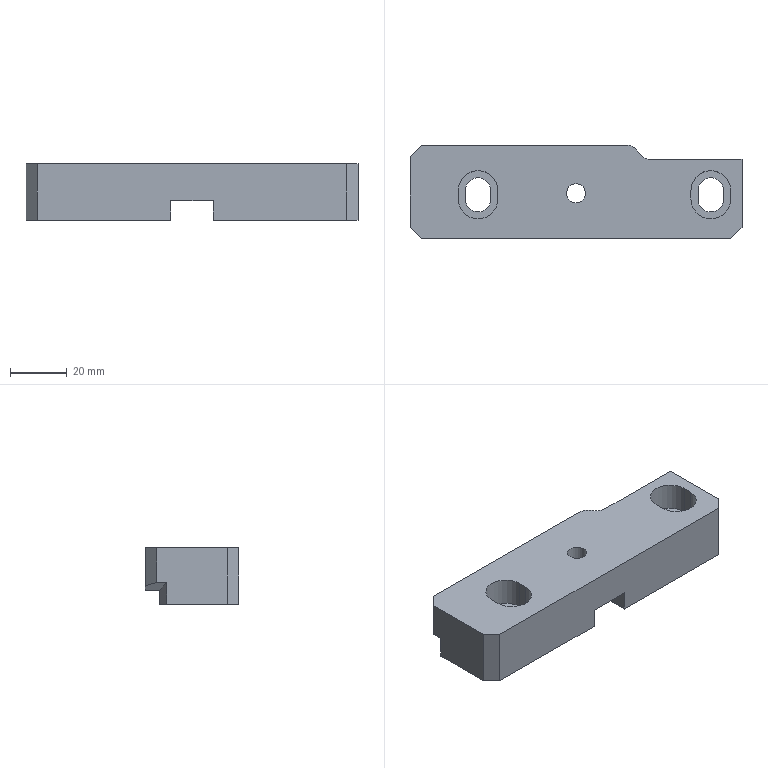Part | NX | features 20 2 | 1 solid | 43 faces | box 117 x 33 x 20 mm | volume 61601 mm3 | plane 32 | cylinder 11 | commonest cylinder face diameters 9 x4 14 x4 10 x2 6.8 x1
STEP:
#1=CARTESIAN_POINT('',(201.002,-436.5,16.5));
#2=VERTEX_POINT('',#1);
#3=CARTESIAN_POINT('',(201.002,-433.5,16.5));
#4=VERTEX_POINT('',#3);
#5=CARTESIAN_POINT('',(201.002,-450.5,16.5));
#6=DIRECTION('',(0.,1.,0.));
#7=VECTOR('',#6,1000.);
#8=LINE('',#5,#7);
#9=EDGE_CURVE('',#2,#4,#8,.T.);
#10=ORIENTED_EDGE('',*,*,#9,.F.);
#11=CARTESIAN_POINT('',(187.002,-436.5,16.5));
#12=VERTEX_POINT('',#11);
#13=CARTESIAN_POINT('',(194.002,-436.5,16.5));
#14=DIRECTION('',(0.,0.,1.));
#15=DIRECTION('',(1.,0.,0.));
#16=AXIS2_PLACEMENT_3D('',#13,#14,#15);
#17=CIRCLE('',#16,7.);
#18=EDGE_CURVE('',#12,#2,#17,.T.);
#19=ORIENTED_EDGE('',*,*,#18,.F.);
#20=CARTESIAN_POINT('',(187.002,-433.5,16.5));
#21=VERTEX_POINT('',#20);
#22=CARTESIAN_POINT('',(187.002,-450.5,16.5));
#23=DIRECTION('',(0.,-1.,0.));
#24=VECTOR('',#23,1000.);
#25=LINE('',#22,#24);
#26=EDGE_CURVE('',#21,#12,#25,.T.);
#27=ORIENTED_EDGE('',*,*,#26,.F.);
#28=CARTESIAN_POINT('',(194.002,-433.5,16.5));
#29=DIRECTION('',(0.,0.,1.));
#30=DIRECTION('',(1.,0.,0.));
#31=AXIS2_PLACEMENT_3D('',#28,#29,#30);
#32=CIRCLE('',#31,7.);
#33=EDGE_CURVE('',#4,#21,#32,.T.);
#34=ORIENTED_EDGE('',*,*,#33,.F.);
#35=EDGE_LOOP('',(#10,#19,#27,#34));
#36=FACE_BOUND('',#35,.T.);
#37=CARTESIAN_POINT('',(283.002,-433.5,16.5));
#38=VERTEX_POINT('',#37);
#39=CARTESIAN_POINT('',(269.002,-433.5,16.5));
#40=VERTEX_POINT('',#39);
#41=CARTESIAN_POINT('',(276.002,-433.5,16.5));
#42=DIRECTION('',(0.,0.,1.));
#43=DIRECTION('',(1.,0.,0.));
#44=AXIS2_PLACEMENT_3D('',#41,#42,#43);
#45=CIRCLE('',#44,7.);
#46=EDGE_CURVE('',#38,#40,#45,.T.);
#47=ORIENTED_EDGE('',*,*,#46,.F.);
#48=CARTESIAN_POINT('',(283.002,-436.5,16.5));
#49=VERTEX_POINT('',#48);
#50=CARTESIAN_POINT('',(283.002,-450.5,16.5));
#51=DIRECTION('',(0.,1.,0.));
#52=VECTOR('',#51,1000.);
#53=LINE('',#50,#52);
#54=EDGE_CURVE('',#49,#38,#53,.T.);
#55=ORIENTED_EDGE('',*,*,#54,.F.);
#56=CARTESIAN_POINT('',(269.002,-436.5,16.5));
#57=VERTEX_POINT('',#56);
#58=CARTESIAN_POINT('',(276.002,-436.5,16.5));
#59=DIRECTION('',(0.,0.,1.));
#60=DIRECTION('',(1.,0.,0.));
#61=AXIS2_PLACEMENT_3D('',#58,#59,#60);
#62=CIRCLE('',#61,7.);
#63=EDGE_CURVE('',#57,#49,#62,.T.);
#64=ORIENTED_EDGE('',*,*,#63,.F.);
#65=CARTESIAN_POINT('',(269.002,-450.5,16.5));
#66=DIRECTION('',(0.,-1.,0.));
#67=VECTOR('',#66,1000.);
#68=LINE('',#65,#67);
#69=EDGE_CURVE('',#40,#57,#68,.T.);
#70=ORIENTED_EDGE('',*,*,#69,.F.);
#71=EDGE_LOOP('',(#47,#55,#64,#70));
#72=FACE_BOUND('',#71,.T.);
#73=CARTESIAN_POINT('',(250.598,-420.,16.5));
#74=VERTEX_POINT('',#73);
#75=CARTESIAN_POINT('',(254.929,-422.5,16.5));
#76=VERTEX_POINT('',#75);
#77=CARTESIAN_POINT('',(254.929,-417.5,16.5));
#78=DIRECTION('',(0.,0.,1.));
#79=DIRECTION('',(1.,0.,0.));
#80=AXIS2_PLACEMENT_3D('',#77,#78,#79);
#81=CIRCLE('',#80,5.);
#82=EDGE_CURVE('',#74,#76,#81,.T.);
#83=ORIENTED_EDGE('',*,*,#82,.F.);
#84=CARTESIAN_POINT('',(246.268,-417.5,16.5));
#85=VERTEX_POINT('',#84);
#86=CARTESIAN_POINT('',(246.268,-422.5,16.5));
#87=DIRECTION('',(0.,0.,1.));
#88=DIRECTION('',(1.,0.,0.));
#89=AXIS2_PLACEMENT_3D('',#86,#87,#88);
#90=CIRCLE('',#89,5.);
#91=EDGE_CURVE('',#74,#85,#90,.T.);
#92=ORIENTED_EDGE('',*,*,#91,.T.);
#93=CARTESIAN_POINT('',(174.002,-417.5,16.5));
#94=VERTEX_POINT('',#93);
#95=CARTESIAN_POINT('',(201.002,-417.5,16.5));
#96=DIRECTION('',(-1.,0.,0.));
#97=VECTOR('',#96,1000.);
#98=LINE('',#95,#97);
#99=EDGE_CURVE('',#85,#94,#98,.T.);
#100=ORIENTED_EDGE('',*,*,#99,.T.);
#101=CARTESIAN_POINT('',(170.002,-421.5,16.5));
#102=VERTEX_POINT('',#101);
#103=CARTESIAN_POINT('',(170.002,-421.5,16.5));
#104=DIRECTION('',(-0.7071,-0.7071,0.));
#105=VECTOR('',#104,1000.);
#106=LINE('',#103,#105);
#107=EDGE_CURVE('',#94,#102,#106,.T.);
#108=ORIENTED_EDGE('',*,*,#107,.T.);
#109=CARTESIAN_POINT('',(170.002,-446.5,16.5));
#110=VERTEX_POINT('',#109);
#111=CARTESIAN_POINT('',(170.002,-417.5,16.5));
#112=DIRECTION('',(0.,-1.,0.));
#113=VECTOR('',#112,1000.);
#114=LINE('',#111,#113);
#115=EDGE_CURVE('',#102,#110,#114,.T.);
#116=ORIENTED_EDGE('',*,*,#115,.T.);
#117=CARTESIAN_POINT('',(174.002,-450.5,16.5));
#118=VERTEX_POINT('',#117);
#119=CARTESIAN_POINT('',(174.002,-450.5,16.5));
#120=DIRECTION('',(0.7071,-0.7071,0.));
#121=VECTOR('',#120,1000.);
#122=LINE('',#119,#121);
#123=EDGE_CURVE('',#110,#118,#122,.T.);
#124=ORIENTED_EDGE('',*,*,#123,.T.);
#125=CARTESIAN_POINT('',(283.002,-450.5,16.5));
#126=VERTEX_POINT('',#125);
#127=CARTESIAN_POINT('',(121.002,-450.5,16.5));
#128=DIRECTION('',(1.,0.,0.));
#129=VECTOR('',#128,1000.);
#130=LINE('',#127,#129);
#131=EDGE_CURVE('',#118,#126,#130,.T.);
#132=ORIENTED_EDGE('',*,*,#131,.T.);
#133=CARTESIAN_POINT('',(287.002,-446.5,16.5));
#134=VERTEX_POINT('',#133);
#135=CARTESIAN_POINT('',(287.002,-446.5,16.5));
#136=DIRECTION('',(0.7071,0.7071,0.));
#137=VECTOR('',#136,1000.);
#138=LINE('',#135,#137);
#139=EDGE_CURVE('',#126,#134,#138,.T.);
#140=ORIENTED_EDGE('',*,*,#139,.T.);
#141=CARTESIAN_POINT('',(287.002,-422.5,16.5));
#142=VERTEX_POINT('',#141);
#143=CARTESIAN_POINT('',(287.002,-450.5,16.5));
#144=DIRECTION('',(0.,1.,0.));
#145=VECTOR('',#144,1000.);
#146=LINE('',#143,#145);
#147=EDGE_CURVE('',#134,#142,#146,.T.);
#148=ORIENTED_EDGE('',*,*,#147,.T.);
#149=CARTESIAN_POINT('',(201.002,-422.5,16.5));
#150=DIRECTION('',(1.,0.,0.));
#151=VECTOR('',#150,1000.);
#152=LINE('',#149,#151);
#153=EDGE_CURVE('',#76,#142,#152,.T.);
#154=ORIENTED_EDGE('',*,*,#153,.F.);
#155=EDGE_LOOP('',(#83,#92,#100,#108,#116,#124,#132,#140,#148,#154));
#156=FACE_BOUND('',#155,.T.);
#157=CARTESIAN_POINT('',(231.902,-434.5,16.5));
#158=VERTEX_POINT('',#157);
#159=CARTESIAN_POINT('',(228.502,-434.5,16.5));
#160=DIRECTION('',(0.,0.,-1.));
#161=DIRECTION('',(1.,0.,0.));
#162=AXIS2_PLACEMENT_3D('',#159,#160,#161);
#163=CIRCLE('',#162,3.4);
#164=EDGE_CURVE('',#158,#158,#163,.T.);
#165=ORIENTED_EDGE('',*,*,#164,.T.);
#166=EDGE_LOOP('',(#165));
#167=FACE_BOUND('',#166,.T.);
#168=CARTESIAN_POINT('',(201.002,-450.5,16.5));
#169=DIRECTION('',(0.,0.,1.));
#170=DIRECTION('',(-1.,0.,0.));
#171=AXIS2_PLACEMENT_3D('',#168,#169,#170);
#172=PLANE('',#171);
#173=ADVANCED_FACE('',(#36,#72,#156,#167),#172,.T.);
#174=CARTESIAN_POINT('',(277.002,-422.5,1.5));
#175=VERTEX_POINT('',#174);
#176=CARTESIAN_POINT('',(277.001,-422.5,1.5));
#177=VERTEX_POINT('',#176);
#178=CARTESIAN_POINT('',(233.273,-422.5,1.5));
#179=DIRECTION('',(-1.,0.,0.));
#180=VECTOR('',#179,1000.);
#181=LINE('',#178,#180);
#182=EDGE_CURVE('',#175,#177,#181,.T.);
#183=ORIENTED_EDGE('',*,*,#182,.F.);
#184=CARTESIAN_POINT('',(277.002,-422.5,1.5));
#185=VERTEX_POINT('',#184);
#186=CARTESIAN_POINT('',(277.002,-425.18,1.5));
#187=DIRECTION('',(0.,-1.,0.));
#188=VECTOR('',#187,1000.);
#189=LINE('',#186,#188);
#190=EDGE_CURVE('',#175,#185,#189,.T.);
#191=ORIENTED_EDGE('',*,*,#190,.T.);
#192=CARTESIAN_POINT('',(287.002,-425.18,1.5));
#193=DIRECTION('',(0.9659,-0.2588,0.));
#194=VECTOR('',#193,1000.);
#195=LINE('',#192,#194);
#196=EDGE_CURVE('',#177,#185,#195,.T.);
#197=ORIENTED_EDGE('',*,*,#196,.F.);
#198=EDGE_LOOP('',(#183,#191,#197));
#199=FACE_BOUND('',#198,.T.);
#200=CARTESIAN_POINT('',(233.273,-396.891,1.5));
#201=DIRECTION('',(0.,0.,-1.));
#202=DIRECTION('',(1.,0.,0.));
#203=AXIS2_PLACEMENT_3D('',#200,#201,#202);
#204=PLANE('',#203);
#205=ADVANCED_FACE('',(#199),#204,.T.);
#206=CARTESIAN_POINT('',(246.268,-417.5,1.5));
#207=VERTEX_POINT('',#206);
#208=CARTESIAN_POINT('',(246.268,-417.5,11.5));
#209=DIRECTION('',(0.,0.,-1.));
#210=VECTOR('',#209,1000.);
#211=LINE('',#208,#210);
#212=EDGE_CURVE('',#85,#207,#211,.T.);
#213=ORIENTED_EDGE('',*,*,#212,.T.);
#214=CARTESIAN_POINT('',(236.002,-417.5,1.5));
#215=VERTEX_POINT('',#214);
#216=CARTESIAN_POINT('',(161.002,-417.5,1.5));
#217=DIRECTION('',(1.,0.,0.));
#218=VECTOR('',#217,1000.);
#219=LINE('',#216,#218);
#220=EDGE_CURVE('',#215,#207,#219,.T.);
#221=ORIENTED_EDGE('',*,*,#220,.F.);
#222=CARTESIAN_POINT('',(236.002,-417.5,3.5));
#223=VERTEX_POINT('',#222);
#224=CARTESIAN_POINT('',(236.002,-417.5,11.5));
#225=DIRECTION('',(0.,0.,-1.));
#226=VECTOR('',#225,1000.);
#227=LINE('',#224,#226);
#228=EDGE_CURVE('',#223,#215,#227,.T.);
#229=ORIENTED_EDGE('',*,*,#228,.F.);
#230=CARTESIAN_POINT('',(221.002,-417.5,3.5));
#231=VERTEX_POINT('',#230);
#232=CARTESIAN_POINT('',(187.002,-417.5,3.5));
#233=DIRECTION('',(1.,0.,0.));
#234=VECTOR('',#233,1000.);
#235=LINE('',#232,#234);
#236=EDGE_CURVE('',#231,#223,#235,.T.);
#237=ORIENTED_EDGE('',*,*,#236,.F.);
#238=CARTESIAN_POINT('',(221.002,-417.5,1.5));
#239=VERTEX_POINT('',#238);
#240=CARTESIAN_POINT('',(221.002,-417.5,-9.5));
#241=DIRECTION('',(0.,0.,1.));
#242=VECTOR('',#241,1000.);
#243=LINE('',#240,#242);
#244=EDGE_CURVE('',#239,#231,#243,.T.);
#245=ORIENTED_EDGE('',*,*,#244,.F.);
#246=CARTESIAN_POINT('',(180.002,-417.5,1.5));
#247=VERTEX_POINT('',#246);
#248=CARTESIAN_POINT('',(201.002,-417.5,1.5));
#249=DIRECTION('',(1.,0.,0.));
#250=VECTOR('',#249,1000.);
#251=LINE('',#248,#250);
#252=EDGE_CURVE('',#247,#239,#251,.T.);
#253=ORIENTED_EDGE('',*,*,#252,.F.);
#254=CARTESIAN_POINT('',(174.002,-417.5,3.108));
#255=VERTEX_POINT('',#254);
#256=CARTESIAN_POINT('',(180.002,-417.5,1.5));
#257=DIRECTION('',(-0.9659,0.,0.2588));
#258=VECTOR('',#257,1000.);
#259=LINE('',#256,#258);
#260=EDGE_CURVE('',#247,#255,#259,.T.);
#261=ORIENTED_EDGE('',*,*,#260,.T.);
#262=CARTESIAN_POINT('',(174.002,-417.5,11.5));
#263=DIRECTION('',(0.,0.,1.));
#264=VECTOR('',#263,1000.);
#265=LINE('',#262,#264);
#266=EDGE_CURVE('',#255,#94,#265,.T.);
#267=ORIENTED_EDGE('',*,*,#266,.T.);
#268=ORIENTED_EDGE('',*,*,#99,.F.);
#269=EDGE_LOOP('',(#213,#221,#229,#237,#245,#253,#261,#267,#268));
#270=FACE_BOUND('',#269,.T.);
#271=CARTESIAN_POINT('',(201.002,-417.5,11.5));
#272=DIRECTION('',(0.,-1.,0.));
#273=DIRECTION('',(0.,0.,1.));
#274=AXIS2_PLACEMENT_3D('',#271,#272,#273);
#275=PLANE('',#274);
#276=ADVANCED_FACE('',(#270),#275,.F.);
#277=CARTESIAN_POINT('',(271.502,-433.5,-3.5));
#278=VERTEX_POINT('',#277);
#279=CARTESIAN_POINT('',(271.502,-436.5,-3.5));
#280=VERTEX_POINT('',#279);
#281=CARTESIAN_POINT('',(271.502,-432.5,-3.5));
#282=DIRECTION('',(0.,-1.,0.));
#283=VECTOR('',#282,1000.);
#284=LINE('',#281,#283);
#285=EDGE_CURVE('',#278,#280,#284,.T.);
#286=ORIENTED_EDGE('',*,*,#285,.T.);
#287=CARTESIAN_POINT('',(280.502,-436.5,-3.5));
#288=VERTEX_POINT('',#287);
#289=CARTESIAN_POINT('',(276.002,-436.5,-3.5));
#290=DIRECTION('',(0.,0.,1.));
#291=DIRECTION('',(1.,0.,0.));
#292=AXIS2_PLACEMENT_3D('',#289,#290,#291);
#293=CIRCLE('',#292,4.5);
#294=EDGE_CURVE('',#280,#288,#293,.T.);
#295=ORIENTED_EDGE('',*,*,#294,.T.);
#296=CARTESIAN_POINT('',(280.502,-433.5,-3.5));
#297=VERTEX_POINT('',#296);
#298=CARTESIAN_POINT('',(280.502,-439.5,-3.5));
#299=DIRECTION('',(0.,1.,0.));
#300=VECTOR('',#299,1000.);
#301=LINE('',#298,#300);
#302=EDGE_CURVE('',#288,#297,#301,.T.);
#303=ORIENTED_EDGE('',*,*,#302,.T.);
#304=CARTESIAN_POINT('',(276.002,-433.5,-3.5));
#305=DIRECTION('',(0.,0.,1.));
#306=DIRECTION('',(1.,0.,0.));
#307=AXIS2_PLACEMENT_3D('',#304,#305,#306);
#308=CIRCLE('',#307,4.5);
#309=EDGE_CURVE('',#297,#278,#308,.T.);
#310=ORIENTED_EDGE('',*,*,#309,.T.);
#311=EDGE_LOOP('',(#286,#295,#303,#310));
#312=FACE_BOUND('',#311,.T.);
#313=CARTESIAN_POINT('',(287.002,-446.5,-3.5));
#314=VERTEX_POINT('',#313);
#315=CARTESIAN_POINT('',(283.002,-450.5,-3.5));
#316=VERTEX_POINT('',#315);
#317=CARTESIAN_POINT('',(287.002,-446.5,-3.5));
#318=DIRECTION('',(-0.7071,-0.7071,0.));
#319=VECTOR('',#318,1000.);
#320=LINE('',#317,#319);
#321=EDGE_CURVE('',#314,#316,#320,.T.);
#322=ORIENTED_EDGE('',*,*,#321,.T.);
#323=CARTESIAN_POINT('',(236.002,-450.5,-3.5));
#324=VERTEX_POINT('',#323);
#325=CARTESIAN_POINT('',(131.002,-450.5,-3.5));
#326=DIRECTION('',(1.,0.,0.));
#327=VECTOR('',#326,1000.);
#328=LINE('',#325,#327);
#329=EDGE_CURVE('',#324,#316,#328,.T.);
#330=ORIENTED_EDGE('',*,*,#329,.F.);
#331=CARTESIAN_POINT('',(236.002,-422.5,-3.5));
#332=VERTEX_POINT('',#331);
#333=CARTESIAN_POINT('',(236.002,-450.5,-3.5));
#334=DIRECTION('',(0.,1.,0.));
#335=VECTOR('',#334,1000.);
#336=LINE('',#333,#335);
#337=EDGE_CURVE('',#324,#332,#336,.T.);
#338=ORIENTED_EDGE('',*,*,#337,.T.);
#339=CARTESIAN_POINT('',(277.001,-422.5,-3.5));
#340=VERTEX_POINT('',#339);
#341=CARTESIAN_POINT('',(201.001,-422.5,-3.5));
#342=DIRECTION('',(-1.,0.,0.));
#343=VECTOR('',#342,1000.);
#344=LINE('',#341,#343);
#345=EDGE_CURVE('',#340,#332,#344,.T.);
#346=ORIENTED_EDGE('',*,*,#345,.F.);
#347=CARTESIAN_POINT('',(287.002,-425.18,-3.5));
#348=VERTEX_POINT('',#347);
#349=CARTESIAN_POINT('',(287.002,-425.18,-3.5));
#350=DIRECTION('',(-0.9659,0.2588,0.));
#351=VECTOR('',#350,1000.);
#352=LINE('',#349,#351);
#353=EDGE_CURVE('',#348,#340,#352,.T.);
#354=ORIENTED_EDGE('',*,*,#353,.F.);
#355=CARTESIAN_POINT('',(287.002,-450.5,-3.5));
#356=DIRECTION('',(0.,1.,0.));
#357=VECTOR('',#356,1000.);
#358=LINE('',#355,#357);
#359=EDGE_CURVE('',#314,#348,#358,.T.);
#360=ORIENTED_EDGE('',*,*,#359,.F.);
#361=EDGE_LOOP('',(#322,#330,#338,#346,#354,#360));
#362=FACE_BOUND('',#361,.T.);
#363=CARTESIAN_POINT('',(151.002,-450.5,-3.5));
#364=DIRECTION('',(0.,0.,1.));
#365=DIRECTION('',(-1.,0.,0.));
#366=AXIS2_PLACEMENT_3D('',#363,#364,#365);
#367=PLANE('',#366);
#368=ADVANCED_FACE('',(#312,#362),#367,.F.);
#369=CARTESIAN_POINT('',(236.002,-422.5,1.5));
#370=VERTEX_POINT('',#369);
#371=CARTESIAN_POINT('',(254.929,-422.5,1.5));
#372=VERTEX_POINT('',#371);
#373=CARTESIAN_POINT('',(183.273,-422.5,1.5));
#374=DIRECTION('',(1.,0.,0.));
#375=VECTOR('',#374,1000.);
#376=LINE('',#373,#375);
#377=EDGE_CURVE('',#370,#372,#376,.T.);
#378=ORIENTED_EDGE('',*,*,#377,.T.);
#379=CARTESIAN_POINT('',(254.929,-422.5,3.5));
#380=DIRECTION('',(0.,0.,-1.));
#381=VECTOR('',#380,1000.);
#382=LINE('',#379,#381);
#383=EDGE_CURVE('',#76,#372,#382,.T.);
#384=ORIENTED_EDGE('',*,*,#383,.F.);
#385=ORIENTED_EDGE('',*,*,#153,.T.);
#386=CARTESIAN_POINT('',(287.002,-422.5,4.179));
#387=VERTEX_POINT('',#386);
#388=CARTESIAN_POINT('',(287.002,-422.5,11.5));
#389=DIRECTION('',(0.,0.,1.));
#390=VECTOR('',#389,1000.);
#391=LINE('',#388,#390);
#392=EDGE_CURVE('',#387,#142,#391,.T.);
#393=ORIENTED_EDGE('',*,*,#392,.F.);
#394=CARTESIAN_POINT('',(277.002,-422.5,1.5));
#395=DIRECTION('',(-0.9659,0.,-0.2588));
#396=VECTOR('',#395,1000.);
#397=LINE('',#394,#396);
#398=EDGE_CURVE('',#387,#175,#397,.T.);
#399=ORIENTED_EDGE('',*,*,#398,.T.);
#400=ORIENTED_EDGE('',*,*,#182,.T.);
#401=CARTESIAN_POINT('',(277.001,-422.5,3.5));
#402=DIRECTION('',(0.,0.,1.));
#403=VECTOR('',#402,1000.);
#404=LINE('',#401,#403);
#405=EDGE_CURVE('',#340,#177,#404,.T.);
#406=ORIENTED_EDGE('',*,*,#405,.F.);
#407=ORIENTED_EDGE('',*,*,#345,.T.);
#408=CARTESIAN_POINT('',(236.002,-422.5,-9.5));
#409=DIRECTION('',(0.,0.,1.));
#410=VECTOR('',#409,1000.);
#411=LINE('',#408,#410);
#412=EDGE_CURVE('',#332,#370,#411,.T.);
#413=ORIENTED_EDGE('',*,*,#412,.T.);
#414=EDGE_LOOP('',(#378,#384,#385,#393,#399,#400,#406,#407,#413));
#415=FACE_BOUND('',#414,.T.);
#416=CARTESIAN_POINT('',(201.001,-422.5,3.5));
#417=DIRECTION('',(0.,-1.,0.));
#418=DIRECTION('',(0.,0.,1.));
#419=AXIS2_PLACEMENT_3D('',#416,#417,#418);
#420=PLANE('',#419);
#421=ADVANCED_FACE('',(#415),#420,.F.);
#422=CARTESIAN_POINT('',(221.002,-422.5,-3.5));
#423=VERTEX_POINT('',#422);
#424=CARTESIAN_POINT('',(221.002,-450.5,-3.5));
#425=VERTEX_POINT('',#424);
#426=CARTESIAN_POINT('',(221.002,-450.5,-3.5));
#427=DIRECTION('',(0.,-1.,0.));
#428=VECTOR('',#427,1000.);
#429=LINE('',#426,#428);
#430=EDGE_CURVE('',#423,#425,#429,.T.);
#431=ORIENTED_EDGE('',*,*,#430,.T.);
#432=CARTESIAN_POINT('',(174.002,-450.5,-3.5));
#433=VERTEX_POINT('',#432);
#434=CARTESIAN_POINT('',(131.002,-450.5,-3.5));
#435=DIRECTION('',(1.,0.,0.));
#436=VECTOR('',#435,1000.);
#437=LINE('',#434,#436);
#438=EDGE_CURVE('',#433,#425,#437,.T.);
#439=ORIENTED_EDGE('',*,*,#438,.F.);
#440=CARTESIAN_POINT('',(170.002,-446.5,-3.5));
#441=VERTEX_POINT('',#440);
#442=CARTESIAN_POINT('',(174.002,-450.5,-3.5));
#443=DIRECTION('',(-0.7071,0.7071,0.));
#444=VECTOR('',#443,1000.);
#445=LINE('',#442,#444);
#446=EDGE_CURVE('',#433,#441,#445,.T.);
#447=ORIENTED_EDGE('',*,*,#446,.T.);
#448=CARTESIAN_POINT('',(170.002,-425.179,-3.5));
#449=VERTEX_POINT('',#448);
#450=CARTESIAN_POINT('',(170.002,-417.5,-3.5));
#451=DIRECTION('',(0.,-1.,0.));
#452=VECTOR('',#451,1000.);
#453=LINE('',#450,#452);
#454=EDGE_CURVE('',#449,#441,#453,.T.);
#455=ORIENTED_EDGE('',*,*,#454,.F.);
#456=CARTESIAN_POINT('',(180.001,-422.5,-3.5));
#457=VERTEX_POINT('',#456);
#458=CARTESIAN_POINT('',(180.001,-422.5,-3.5));
#459=DIRECTION('',(-0.9659,-0.2588,0.));
#460=VECTOR('',#459,1000.);
#461=LINE('',#458,#460);
#462=EDGE_CURVE('',#457,#449,#461,.T.);
#463=ORIENTED_EDGE('',*,*,#462,.F.);
#464=CARTESIAN_POINT('',(191.001,-422.5,-3.5));
#465=DIRECTION('',(-1.,0.,0.));
#466=VECTOR('',#465,1000.);
#467=LINE('',#464,#466);
#468=EDGE_CURVE('',#423,#457,#467,.T.);
#469=ORIENTED_EDGE('',*,*,#468,.F.);
#470=EDGE_LOOP('',(#431,#439,#447,#455,#463,#469));
#471=FACE_BOUND('',#470,.T.);
#472=CARTESIAN_POINT('',(198.502,-433.5,-3.5));
#473=VERTEX_POINT('',#472);
#474=CARTESIAN_POINT('',(198.502,-436.5,-3.5));
#475=VERTEX_POINT('',#474);
#476=CARTESIAN_POINT('',(198.502,-450.5,-3.5));
#477=DIRECTION('',(0.,-1.,0.));
#478=VECTOR('',#477,1000.);
#479=LINE('',#476,#478);
#480=EDGE_CURVE('',#473,#475,#479,.T.);
#481=ORIENTED_EDGE('',*,*,#480,.F.);
#482=CARTESIAN_POINT('',(189.502,-433.5,-3.5));
#483=VERTEX_POINT('',#482);
#484=CARTESIAN_POINT('',(194.002,-433.5,-3.5));
#485=DIRECTION('',(0.,0.,-1.));
#486=DIRECTION('',(1.,0.,0.));
#487=AXIS2_PLACEMENT_3D('',#484,#485,#486);
#488=CIRCLE('',#487,4.5);
#489=EDGE_CURVE('',#483,#473,#488,.T.);
#490=ORIENTED_EDGE('',*,*,#489,.F.);
#491=CARTESIAN_POINT('',(189.502,-436.5,-3.5));
#492=VERTEX_POINT('',#491);
#493=CARTESIAN_POINT('',(189.502,-450.5,-3.5));
#494=DIRECTION('',(0.,1.,0.));
#495=VECTOR('',#494,1000.);
#496=LINE('',#493,#495);
#497=EDGE_CURVE('',#492,#483,#496,.T.);
#498=ORIENTED_EDGE('',*,*,#497,.F.);
#499=CARTESIAN_POINT('',(194.002,-436.5,-3.5));
#500=DIRECTION('',(0.,0.,-1.));
#501=DIRECTION('',(1.,0.,0.));
#502=AXIS2_PLACEMENT_3D('',#499,#500,#501);
#503=CIRCLE('',#502,4.5);
#504=EDGE_CURVE('',#475,#492,#503,.T.);
#505=ORIENTED_EDGE('',*,*,#504,.F.);
#506=EDGE_LOOP('',(#481,#490,#498,#505));
#507=FACE_BOUND('',#506,.T.);
#508=CARTESIAN_POINT('',(201.002,-450.5,-3.5));
#509=DIRECTION('',(0.,0.,1.));
#510=DIRECTION('',(-1.,0.,0.));
#511=AXIS2_PLACEMENT_3D('',#508,#509,#510);
#512=PLANE('',#511);
#513=ADVANCED_FACE('',(#471,#507),#512,.F.);
#514=ORIENTED_EDGE('',*,*,#398,.F.);
#515=CARTESIAN_POINT('',(287.002,-425.18,4.179));
#516=VERTEX_POINT('',#515);
#517=CARTESIAN_POINT('',(287.002,-417.5,4.179));
#518=DIRECTION('',(0.,1.,0.));
#519=VECTOR('',#518,1000.);
#520=LINE('',#517,#519);
#521=EDGE_CURVE('',#516,#387,#520,.T.);
#522=ORIENTED_EDGE('',*,*,#521,.F.);
#523=CARTESIAN_POINT('',(286.375,-425.012,4.011));
#524=DIRECTION('',(0.9351,-0.2506,0.2506));
#525=VECTOR('',#524,1000.);
#526=LINE('',#523,#525);
#527=EDGE_CURVE('',#185,#516,#526,.T.);
#528=ORIENTED_EDGE('',*,*,#527,.F.);
#529=ORIENTED_EDGE('',*,*,#190,.F.);
#530=EDGE_LOOP('',(#514,#522,#528,#529));
#531=FACE_BOUND('',#530,.T.);
#532=CARTESIAN_POINT('',(277.002,-396.891,1.5));
#533=DIRECTION('',(0.2588,0.,-0.9659));
#534=DIRECTION('',(0.9659,0.,0.2588));
#535=AXIS2_PLACEMENT_3D('',#532,#533,#534);
#536=PLANE('',#535);
#537=ADVANCED_FACE('',(#531),#536,.T.);
#538=ORIENTED_EDGE('',*,*,#220,.T.);
#539=CARTESIAN_POINT('',(250.598,-420.,1.5));
#540=VERTEX_POINT('',#539);
#541=CARTESIAN_POINT('',(246.268,-422.5,1.5));
#542=DIRECTION('',(0.,0.,-1.));
#543=DIRECTION('',(-1.,0.,0.));
#544=AXIS2_PLACEMENT_3D('',#541,#542,#543);
#545=CIRCLE('',#544,5.);
#546=EDGE_CURVE('',#207,#540,#545,.T.);
#547=ORIENTED_EDGE('',*,*,#546,.T.);
#548=CARTESIAN_POINT('',(254.929,-417.5,1.5));
#549=DIRECTION('',(0.,0.,1.));
#550=DIRECTION('',(-1.,0.,0.));
#551=AXIS2_PLACEMENT_3D('',#548,#549,#550);
#552=CIRCLE('',#551,5.);
#553=EDGE_CURVE('',#540,#372,#552,.T.);
#554=ORIENTED_EDGE('',*,*,#553,.T.);
#555=ORIENTED_EDGE('',*,*,#377,.F.);
#556=CARTESIAN_POINT('',(236.002,-436.5,1.5));
#557=DIRECTION('',(0.,1.,0.));
#558=VECTOR('',#557,1000.);
#559=LINE('',#556,#558);
#560=EDGE_CURVE('',#370,#215,#559,.T.);
#561=ORIENTED_EDGE('',*,*,#560,.T.);
#562=EDGE_LOOP('',(#538,#547,#554,#555,#561));
#563=FACE_BOUND('',#562,.T.);
#564=CARTESIAN_POINT('',(233.273,-396.891,1.5));
#565=DIRECTION('',(0.,0.,-1.));
#566=DIRECTION('',(1.,0.,0.));
#567=AXIS2_PLACEMENT_3D('',#564,#565,#566);
#568=PLANE('',#567);
#569=ADVANCED_FACE('',(#563),#568,.T.);
#570=CARTESIAN_POINT('',(170.002,-421.5,4.179));
#571=VERTEX_POINT('',#570);
#572=CARTESIAN_POINT('',(170.002,-425.179,4.179));
#573=VERTEX_POINT('',#572);
#574=CARTESIAN_POINT('',(170.002,-425.179,4.179));
#575=DIRECTION('',(0.,-1.,0.));
#576=VECTOR('',#575,1000.);
#577=LINE('',#574,#576);
#578=EDGE_CURVE('',#571,#573,#577,.T.);
#579=ORIENTED_EDGE('',*,*,#578,.F.);
#580=CARTESIAN_POINT('',(187.054,-404.449,-0.3894));
#581=DIRECTION('',(0.6947,0.6947,-0.1862));
#582=VECTOR('',#581,1000.);
#583=LINE('',#580,#582);
#584=EDGE_CURVE('',#571,#255,#583,.T.);
#585=ORIENTED_EDGE('',*,*,#584,.T.);
#586=ORIENTED_EDGE('',*,*,#260,.F.);
#587=CARTESIAN_POINT('',(180.002,-422.5,1.5));
#588=VERTEX_POINT('',#587);
#589=CARTESIAN_POINT('',(180.002,-417.5,1.5));
#590=DIRECTION('',(0.,1.,0.));
#591=VECTOR('',#590,1000.);
#592=LINE('',#589,#591);
#593=EDGE_CURVE('',#588,#247,#592,.T.);
#594=ORIENTED_EDGE('',*,*,#593,.F.);
#595=CARTESIAN_POINT('',(180.001,-422.5,1.5));
#596=VERTEX_POINT('',#595);
#597=CARTESIAN_POINT('',(180.002,-422.5,1.5));
#598=DIRECTION('',(0.9659,0.,-0.2588));
#599=VECTOR('',#598,1000.);
#600=LINE('',#597,#599);
#601=EDGE_CURVE('',#596,#588,#600,.T.);
#602=ORIENTED_EDGE('',*,*,#601,.F.);
#603=CARTESIAN_POINT('',(180.001,-422.5,1.5));
#604=DIRECTION('',(0.9351,0.2506,-0.2506));
#605=VECTOR('',#604,1000.);
#606=LINE('',#603,#605);
#607=EDGE_CURVE('',#573,#596,#606,.T.);
#608=ORIENTED_EDGE('',*,*,#607,.F.);
#609=EDGE_LOOP('',(#579,#585,#586,#594,#602,#608));
#610=FACE_BOUND('',#609,.T.);
#611=CARTESIAN_POINT('',(180.002,-396.891,1.5));
#612=DIRECTION('',(-0.2588,0.,-0.9659));
#613=DIRECTION('',(0.9659,0.,-0.2588));
#614=AXIS2_PLACEMENT_3D('',#611,#612,#613);
#615=PLANE('',#614);
#616=ADVANCED_FACE('',(#610),#615,.T.);
#617=ORIENTED_EDGE('',*,*,#521,.T.);
#618=ORIENTED_EDGE('',*,*,#392,.T.);
#619=ORIENTED_EDGE('',*,*,#147,.F.);
#620=CARTESIAN_POINT('',(287.002,-446.5,11.5));
#621=DIRECTION('',(0.,0.,-1.));
#622=VECTOR('',#621,1000.);
#623=LINE('',#620,#622);
#624=EDGE_CURVE('',#134,#314,#623,.T.);
#625=ORIENTED_EDGE('',*,*,#624,.T.);
#626=ORIENTED_EDGE('',*,*,#359,.T.);
#627=CARTESIAN_POINT('',(287.002,-425.18,3.5));
#628=DIRECTION('',(0.,0.,-1.));
#629=VECTOR('',#628,1000.);
#630=LINE('',#627,#629);
#631=EDGE_CURVE('',#516,#348,#630,.T.);
#632=ORIENTED_EDGE('',*,*,#631,.F.);
#633=EDGE_LOOP('',(#617,#618,#619,#625,#626,#632));
#634=FACE_BOUND('',#633,.T.);
#635=CARTESIAN_POINT('',(287.002,-450.5,11.5));
#636=DIRECTION('',(-1.,0.,0.));
#637=DIRECTION('',(0.,0.,-1.));
#638=AXIS2_PLACEMENT_3D('',#635,#636,#637);
#639=PLANE('',#638);
#640=ADVANCED_FACE('',(#634),#639,.F.);
#641=ORIENTED_EDGE('',*,*,#115,.F.);
#642=CARTESIAN_POINT('',(170.002,-421.5,11.5));
#643=DIRECTION('',(0.,0.,-1.));
#644=VECTOR('',#643,1000.);
#645=LINE('',#642,#644);
#646=EDGE_CURVE('',#102,#571,#645,.T.);
#647=ORIENTED_EDGE('',*,*,#646,.T.);
#648=ORIENTED_EDGE('',*,*,#578,.T.);
#649=CARTESIAN_POINT('',(170.002,-425.179,3.5));
#650=DIRECTION('',(0.,0.,-1.));
#651=VECTOR('',#650,1000.);
#652=LINE('',#649,#651);
#653=EDGE_CURVE('',#573,#449,#652,.T.);
#654=ORIENTED_EDGE('',*,*,#653,.T.);
#655=ORIENTED_EDGE('',*,*,#454,.T.);
#656=CARTESIAN_POINT('',(170.002,-446.5,11.5));
#657=DIRECTION('',(0.,0.,1.));
#658=VECTOR('',#657,1000.);
#659=LINE('',#656,#658);
#660=EDGE_CURVE('',#441,#110,#659,.T.);
#661=ORIENTED_EDGE('',*,*,#660,.T.);
#662=EDGE_LOOP('',(#641,#647,#648,#654,#655,#661));
#663=FACE_BOUND('',#662,.T.);
#664=CARTESIAN_POINT('',(170.002,-417.5,11.5));
#665=DIRECTION('',(1.,0.,0.));
#666=DIRECTION('',(0.,0.,1.));
#667=AXIS2_PLACEMENT_3D('',#664,#665,#666);
#668=PLANE('',#667);
#669=ADVANCED_FACE('',(#663),#668,.F.);
#670=CARTESIAN_POINT('',(271.502,-433.5,6.5));
#671=VERTEX_POINT('',#670);
#672=CARTESIAN_POINT('',(280.502,-433.5,6.5));
#673=VERTEX_POINT('',#672);
#674=CARTESIAN_POINT('',(276.002,-433.5,6.5));
#675=DIRECTION('',(0.,0.,-1.));
#676=DIRECTION('',(-1.,0.,0.));
#677=AXIS2_PLACEMENT_3D('',#674,#675,#676);
#678=CIRCLE('',#677,4.5);
#679=EDGE_CURVE('',#671,#673,#678,.T.);
#680=ORIENTED_EDGE('',*,*,#679,.F.);
#681=CARTESIAN_POINT('',(271.502,-433.5,42.5));
#682=DIRECTION('',(0.,0.,1.));
#683=VECTOR('',#682,1000.);
#684=LINE('',#681,#683);
#685=EDGE_CURVE('',#278,#671,#684,.T.);
#686=ORIENTED_EDGE('',*,*,#685,.F.);
#687=ORIENTED_EDGE('',*,*,#309,.F.);
#688=CARTESIAN_POINT('',(280.502,-433.5,42.5));
#689=DIRECTION('',(0.,0.,1.));
#690=VECTOR('',#689,1000.);
#691=LINE('',#688,#690);
#692=EDGE_CURVE('',#297,#673,#691,.T.);
#693=ORIENTED_EDGE('',*,*,#692,.T.);
#694=EDGE_LOOP('',(#680,#686,#687,#693));
#695=FACE_BOUND('',#694,.T.);
#696=CARTESIAN_POINT('',(276.002,-433.5,42.5));
#697=DIRECTION('',(0.,0.,-1.));
#698=DIRECTION('',(1.,0.,0.));
#699=AXIS2_PLACEMENT_3D('',#696,#697,#698);
#700=CYLINDRICAL_SURFACE('',#699,4.5);
#701=ADVANCED_FACE('',(#695),#700,.F.);
#702=CARTESIAN_POINT('',(280.502,-436.5,6.5));
#703=VERTEX_POINT('',#702);
#704=CARTESIAN_POINT('',(280.502,-439.5,6.5));
#705=DIRECTION('',(0.,-1.,0.));
#706=VECTOR('',#705,1000.);
#707=LINE('',#704,#706);
#708=EDGE_CURVE('',#673,#703,#707,.T.);
#709=ORIENTED_EDGE('',*,*,#708,.F.);
#710=ORIENTED_EDGE('',*,*,#692,.F.);
#711=ORIENTED_EDGE('',*,*,#302,.F.);
#712=CARTESIAN_POINT('',(280.502,-436.5,42.5));
#713=DIRECTION('',(0.,0.,1.));
#714=VECTOR('',#713,1000.);
#715=LINE('',#712,#714);
#716=EDGE_CURVE('',#288,#703,#715,.T.);
#717=ORIENTED_EDGE('',*,*,#716,.T.);
#718=EDGE_LOOP('',(#709,#710,#711,#717));
#719=FACE_BOUND('',#718,.T.);
#720=CARTESIAN_POINT('',(280.502,-439.5,42.5));
#721=DIRECTION('',(-1.,0.,0.));
#722=DIRECTION('',(0.,0.,-1.));
#723=AXIS2_PLACEMENT_3D('',#720,#721,#722);
#724=PLANE('',#723);
#725=ADVANCED_FACE('',(#719),#724,.T.);
#726=CARTESIAN_POINT('',(271.502,-436.5,6.5));
#727=VERTEX_POINT('',#726);
#728=CARTESIAN_POINT('',(276.002,-436.5,6.5));
#729=DIRECTION('',(0.,0.,-1.));
#730=DIRECTION('',(-1.,0.,0.));
#731=AXIS2_PLACEMENT_3D('',#728,#729,#730);
#732=CIRCLE('',#731,4.5);
#733=EDGE_CURVE('',#703,#727,#732,.T.);
#734=ORIENTED_EDGE('',*,*,#733,.F.);
#735=ORIENTED_EDGE('',*,*,#716,.F.);
#736=ORIENTED_EDGE('',*,*,#294,.F.);
#737=CARTESIAN_POINT('',(271.502,-436.5,42.5));
#738=DIRECTION('',(0.,0.,1.));
#739=VECTOR('',#738,1000.);
#740=LINE('',#737,#739);
#741=EDGE_CURVE('',#280,#727,#740,.T.);
#742=ORIENTED_EDGE('',*,*,#741,.T.);
#743=EDGE_LOOP('',(#734,#735,#736,#742));
#744=FACE_BOUND('',#743,.T.);
#745=CARTESIAN_POINT('',(276.002,-436.5,42.5));
#746=DIRECTION('',(0.,0.,-1.));
#747=DIRECTION('',(1.,0.,0.));
#748=AXIS2_PLACEMENT_3D('',#745,#746,#747);
#749=CYLINDRICAL_SURFACE('',#748,4.5);
#750=ADVANCED_FACE('',(#744),#749,.F.);
#751=CARTESIAN_POINT('',(271.502,-432.5,6.5));
#752=DIRECTION('',(0.,1.,0.));
#753=VECTOR('',#752,1000.);
#754=LINE('',#751,#753);
#755=EDGE_CURVE('',#727,#671,#754,.T.);
#756=ORIENTED_EDGE('',*,*,#755,.F.);
#757=ORIENTED_EDGE('',*,*,#741,.F.);
#758=ORIENTED_EDGE('',*,*,#285,.F.);
#759=ORIENTED_EDGE('',*,*,#685,.T.);
#760=EDGE_LOOP('',(#756,#757,#758,#759));
#761=FACE_BOUND('',#760,.T.);
#762=CARTESIAN_POINT('',(271.502,-432.5,42.5));
#763=DIRECTION('',(1.,0.,0.));
#764=DIRECTION('',(0.,0.,1.));
#765=AXIS2_PLACEMENT_3D('',#762,#763,#764);
#766=PLANE('',#765);
#767=ADVANCED_FACE('',(#761),#766,.T.);
#768=ORIENTED_EDGE('',*,*,#755,.T.);
#769=ORIENTED_EDGE('',*,*,#679,.T.);
#770=ORIENTED_EDGE('',*,*,#708,.T.);
#771=ORIENTED_EDGE('',*,*,#733,.T.);
#772=EDGE_LOOP('',(#768,#769,#770,#771));
#773=FACE_BOUND('',#772,.T.);
#774=CARTESIAN_POINT('',(283.002,-433.5,6.5));
#775=VERTEX_POINT('',#774);
#776=CARTESIAN_POINT('',(269.002,-433.5,6.5));
#777=VERTEX_POINT('',#776);
#778=CARTESIAN_POINT('',(276.002,-433.5,6.5));
#779=DIRECTION('',(0.,0.,1.));
#780=DIRECTION('',(-1.,0.,0.));
#781=AXIS2_PLACEMENT_3D('',#778,#779,#780);
#782=CIRCLE('',#781,7.);
#783=EDGE_CURVE('',#775,#777,#782,.T.);
#784=ORIENTED_EDGE('',*,*,#783,.T.);
#785=CARTESIAN_POINT('',(269.002,-436.5,6.5));
#786=VERTEX_POINT('',#785);
#787=CARTESIAN_POINT('',(269.002,-439.5,6.5));
#788=DIRECTION('',(0.,-1.,0.));
#789=VECTOR('',#788,1000.);
#790=LINE('',#787,#789);
#791=EDGE_CURVE('',#777,#786,#790,.T.);
#792=ORIENTED_EDGE('',*,*,#791,.T.);
#793=CARTESIAN_POINT('',(283.002,-436.5,6.5));
#794=VERTEX_POINT('',#793);
#795=CARTESIAN_POINT('',(276.002,-436.5,6.5));
#796=DIRECTION('',(0.,0.,1.));
#797=DIRECTION('',(-1.,0.,0.));
#798=AXIS2_PLACEMENT_3D('',#795,#796,#797);
#799=CIRCLE('',#798,7.);
#800=EDGE_CURVE('',#786,#794,#799,.T.);
#801=ORIENTED_EDGE('',*,*,#800,.T.);
#802=CARTESIAN_POINT('',(283.002,-432.5,6.5));
#803=DIRECTION('',(0.,1.,0.));
#804=VECTOR('',#803,1000.);
#805=LINE('',#802,#804);
#806=EDGE_CURVE('',#794,#775,#805,.T.);
#807=ORIENTED_EDGE('',*,*,#806,.T.);
#808=EDGE_LOOP('',(#784,#792,#801,#807));
#809=FACE_BOUND('',#808,.T.);
#810=CARTESIAN_POINT('',(276.002,-432.5,6.5));
#811=DIRECTION('',(0.,0.,-1.));
#812=DIRECTION('',(1.,0.,0.));
#813=AXIS2_PLACEMENT_3D('',#810,#811,#812);
#814=PLANE('',#813);
#815=ADVANCED_FACE('',(#773,#809),#814,.F.);
#816=ORIENTED_EDGE('',*,*,#196,.T.);
#817=ORIENTED_EDGE('',*,*,#527,.T.);
#818=ORIENTED_EDGE('',*,*,#631,.T.);
#819=ORIENTED_EDGE('',*,*,#353,.T.);
#820=ORIENTED_EDGE('',*,*,#405,.T.);
#821=EDGE_LOOP('',(#816,#817,#818,#819,#820));
#822=FACE_BOUND('',#821,.T.);
#823=CARTESIAN_POINT('',(287.002,-425.18,3.5));
#824=DIRECTION('',(-0.2588,-0.9659,0.));
#825=DIRECTION('',(0.9659,-0.2588,0.));
#826=AXIS2_PLACEMENT_3D('',#823,#824,#825);
#827=PLANE('',#826);
#828=ADVANCED_FACE('',(#822),#827,.F.);
#829=CARTESIAN_POINT('',(198.502,-433.5,6.5));
#830=VERTEX_POINT('',#829);
#831=CARTESIAN_POINT('',(198.502,-436.5,6.5));
#832=VERTEX_POINT('',#831);
#833=CARTESIAN_POINT('',(198.502,-432.5,6.5));
#834=DIRECTION('',(0.,-1.,0.));
#835=VECTOR('',#834,1000.);
#836=LINE('',#833,#835);
#837=EDGE_CURVE('',#830,#832,#836,.T.);
#838=ORIENTED_EDGE('',*,*,#837,.T.);
#839=CARTESIAN_POINT('',(189.502,-436.5,6.5));
#840=VERTEX_POINT('',#839);
#841=CARTESIAN_POINT('',(194.002,-436.5,6.5));
#842=DIRECTION('',(0.,0.,-1.));
#843=DIRECTION('',(-1.,0.,0.));
#844=AXIS2_PLACEMENT_3D('',#841,#842,#843);
#845=CIRCLE('',#844,4.5);
#846=EDGE_CURVE('',#832,#840,#845,.T.);
#847=ORIENTED_EDGE('',*,*,#846,.T.);
#848=CARTESIAN_POINT('',(189.502,-433.5,6.5));
#849=VERTEX_POINT('',#848);
#850=CARTESIAN_POINT('',(189.502,-439.5,6.5));
#851=DIRECTION('',(0.,1.,0.));
#852=VECTOR('',#851,1000.);
#853=LINE('',#850,#852);
#854=EDGE_CURVE('',#840,#849,#853,.T.);
#855=ORIENTED_EDGE('',*,*,#854,.T.);
#856=CARTESIAN_POINT('',(194.002,-433.5,6.5));
#857=DIRECTION('',(0.,0.,-1.));
#858=DIRECTION('',(-1.,0.,0.));
#859=AXIS2_PLACEMENT_3D('',#856,#857,#858);
#860=CIRCLE('',#859,4.5);
#861=EDGE_CURVE('',#849,#830,#860,.T.);
#862=ORIENTED_EDGE('',*,*,#861,.T.);
#863=EDGE_LOOP('',(#838,#847,#855,#862));
#864=FACE_BOUND('',#863,.T.);
#865=CARTESIAN_POINT('',(201.002,-433.5,6.5));
#866=VERTEX_POINT('',#865);
#867=CARTESIAN_POINT('',(187.002,-433.5,6.5));
#868=VERTEX_POINT('',#867);
#869=CARTESIAN_POINT('',(194.002,-433.5,6.5));
#870=DIRECTION('',(0.,0.,1.));
#871=DIRECTION('',(-1.,0.,0.));
#872=AXIS2_PLACEMENT_3D('',#869,#870,#871);
#873=CIRCLE('',#872,7.);
#874=EDGE_CURVE('',#866,#868,#873,.T.);
#875=ORIENTED_EDGE('',*,*,#874,.T.);
#876=CARTESIAN_POINT('',(187.002,-436.5,6.5));
#877=VERTEX_POINT('',#876);
#878=CARTESIAN_POINT('',(187.002,-432.5,6.5));
#879=DIRECTION('',(0.,-1.,0.));
#880=VECTOR('',#879,1000.);
#881=LINE('',#878,#880);
#882=EDGE_CURVE('',#868,#877,#881,.T.);
#883=ORIENTED_EDGE('',*,*,#882,.T.);
#884=CARTESIAN_POINT('',(201.002,-436.5,6.5));
#885=VERTEX_POINT('',#884);
#886=CARTESIAN_POINT('',(194.002,-436.5,6.5));
#887=DIRECTION('',(0.,0.,1.));
#888=DIRECTION('',(-1.,0.,0.));
#889=AXIS2_PLACEMENT_3D('',#886,#887,#888);
#890=CIRCLE('',#889,7.);
#891=EDGE_CURVE('',#877,#885,#890,.T.);
#892=ORIENTED_EDGE('',*,*,#891,.T.);
#893=CARTESIAN_POINT('',(201.002,-439.5,6.5));
#894=DIRECTION('',(0.,1.,0.));
#895=VECTOR('',#894,1000.);
#896=LINE('',#893,#895);
#897=EDGE_CURVE('',#885,#866,#896,.T.);
#898=ORIENTED_EDGE('',*,*,#897,.T.);
#899=EDGE_LOOP('',(#875,#883,#892,#898));
#900=FACE_BOUND('',#899,.T.);
#901=CARTESIAN_POINT('',(194.002,-432.5,6.5));
#902=DIRECTION('',(0.,0.,-1.));
#903=DIRECTION('',(-1.,0.,0.));
#904=AXIS2_PLACEMENT_3D('',#901,#902,#903);
#905=PLANE('',#904);
#906=ADVANCED_FACE('',(#864,#900),#905,.F.);
#907=ORIENTED_EDGE('',*,*,#69,.T.);
#908=CARTESIAN_POINT('',(269.002,-436.5,42.5));
#909=DIRECTION('',(0.,0.,1.));
#910=VECTOR('',#909,1000.);
#911=LINE('',#908,#910);
#912=EDGE_CURVE('',#786,#57,#911,.T.);
#913=ORIENTED_EDGE('',*,*,#912,.F.);
#914=ORIENTED_EDGE('',*,*,#791,.F.);
#915=CARTESIAN_POINT('',(269.002,-433.5,42.5));
#916=DIRECTION('',(0.,0.,1.));
#917=VECTOR('',#916,1000.);
#918=LINE('',#915,#917);
#919=EDGE_CURVE('',#777,#40,#918,.T.);
#920=ORIENTED_EDGE('',*,*,#919,.T.);
#921=EDGE_LOOP('',(#907,#913,#914,#920));
#922=FACE_BOUND('',#921,.T.);
#923=CARTESIAN_POINT('',(269.002,-439.5,42.5));
#924=DIRECTION('',(-1.,0.,0.));
#925=DIRECTION('',(0.,0.,-1.));
#926=AXIS2_PLACEMENT_3D('',#923,#924,#925);
#927=PLANE('',#926);
#928=ADVANCED_FACE('',(#922),#927,.F.);
#929=ORIENTED_EDGE('',*,*,#63,.T.);
#930=CARTESIAN_POINT('',(283.002,-436.5,42.5));
#931=DIRECTION('',(0.,0.,1.));
#932=VECTOR('',#931,1000.);
#933=LINE('',#930,#932);
#934=EDGE_CURVE('',#794,#49,#933,.T.);
#935=ORIENTED_EDGE('',*,*,#934,.F.);
#936=ORIENTED_EDGE('',*,*,#800,.F.);
#937=ORIENTED_EDGE('',*,*,#912,.T.);
#938=EDGE_LOOP('',(#929,#935,#936,#937));
#939=FACE_BOUND('',#938,.T.);
#940=CARTESIAN_POINT('',(276.002,-436.5,42.5));
#941=DIRECTION('',(0.,0.,-1.));
#942=DIRECTION('',(1.,0.,0.));
#943=AXIS2_PLACEMENT_3D('',#940,#941,#942);
#944=CYLINDRICAL_SURFACE('',#943,7.);
#945=ADVANCED_FACE('',(#939),#944,.F.);
#946=ORIENTED_EDGE('',*,*,#54,.T.);
#947=CARTESIAN_POINT('',(283.002,-433.5,42.5));
#948=DIRECTION('',(0.,0.,1.));
#949=VECTOR('',#948,1000.);
#950=LINE('',#947,#949);
#951=EDGE_CURVE('',#775,#38,#950,.T.);
#952=ORIENTED_EDGE('',*,*,#951,.F.);
#953=ORIENTED_EDGE('',*,*,#806,.F.);
#954=ORIENTED_EDGE('',*,*,#934,.T.);
#955=EDGE_LOOP('',(#946,#952,#953,#954));
#956=FACE_BOUND('',#955,.T.);
#957=CARTESIAN_POINT('',(283.002,-432.5,42.5));
#958=DIRECTION('',(1.,0.,0.));
#959=DIRECTION('',(0.,0.,1.));
#960=AXIS2_PLACEMENT_3D('',#957,#958,#959);
#961=PLANE('',#960);
#962=ADVANCED_FACE('',(#956),#961,.F.);
#963=ORIENTED_EDGE('',*,*,#46,.T.);
#964=ORIENTED_EDGE('',*,*,#919,.F.);
#965=ORIENTED_EDGE('',*,*,#783,.F.);
#966=ORIENTED_EDGE('',*,*,#951,.T.);
#967=EDGE_LOOP('',(#963,#964,#965,#966));
#968=FACE_BOUND('',#967,.T.);
#969=CARTESIAN_POINT('',(276.002,-433.5,42.5));
#970=DIRECTION('',(0.,0.,-1.));
#971=DIRECTION('',(1.,0.,0.));
#972=AXIS2_PLACEMENT_3D('',#969,#970,#971);
#973=CYLINDRICAL_SURFACE('',#972,7.);
#974=ADVANCED_FACE('',(#968),#973,.F.);
#975=ORIENTED_EDGE('',*,*,#321,.F.);
#976=ORIENTED_EDGE('',*,*,#624,.F.);
#977=ORIENTED_EDGE('',*,*,#139,.F.);
#978=CARTESIAN_POINT('',(283.002,-450.5,11.5));
#979=DIRECTION('',(0.,0.,1.));
#980=VECTOR('',#979,1000.);
#981=LINE('',#978,#980);
#982=EDGE_CURVE('',#316,#126,#981,.T.);
#983=ORIENTED_EDGE('',*,*,#982,.F.);
#984=EDGE_LOOP('',(#975,#976,#977,#983));
#985=FACE_BOUND('',#984,.T.);
#986=CARTESIAN_POINT('',(287.002,-446.5,11.5));
#987=DIRECTION('',(-0.7071,0.7071,0.));
#988=DIRECTION('',(0.,0.,-1.));
#989=AXIS2_PLACEMENT_3D('',#986,#987,#988);
#990=PLANE('',#989);
#991=ADVANCED_FACE('',(#985),#990,.F.);
#992=ORIENTED_EDGE('',*,*,#462,.T.);
#993=ORIENTED_EDGE('',*,*,#653,.F.);
#994=ORIENTED_EDGE('',*,*,#607,.T.);
#995=CARTESIAN_POINT('',(180.001,-422.5,3.5));
#996=DIRECTION('',(0.,0.,1.));
#997=VECTOR('',#996,1000.);
#998=LINE('',#995,#997);
#999=EDGE_CURVE('',#457,#596,#998,.T.);
#1000=ORIENTED_EDGE('',*,*,#999,.F.);
#1001=EDGE_LOOP('',(#992,#993,#994,#1000));
#1002=FACE_BOUND('',#1001,.T.);
#1003=CARTESIAN_POINT('',(180.001,-422.5,3.5));
#1004=DIRECTION('',(0.2588,-0.9659,0.));
#1005=DIRECTION('',(0.9659,0.2588,0.));
#1006=AXIS2_PLACEMENT_3D('',#1003,#1004,#1005);
#1007=PLANE('',#1006);
#1008=ADVANCED_FACE('',(#1002),#1007,.F.);
#1009=ORIENTED_EDGE('',*,*,#446,.F.);
#1010=CARTESIAN_POINT('',(174.002,-450.5,11.5));
#1011=DIRECTION('',(0.,0.,-1.));
#1012=VECTOR('',#1011,1000.);
#1013=LINE('',#1010,#1012);
#1014=EDGE_CURVE('',#118,#433,#1013,.T.);
#1015=ORIENTED_EDGE('',*,*,#1014,.F.);
#1016=ORIENTED_EDGE('',*,*,#123,.F.);
#1017=ORIENTED_EDGE('',*,*,#660,.F.);
#1018=EDGE_LOOP('',(#1009,#1015,#1016,#1017));
#1019=FACE_BOUND('',#1018,.T.);
#1020=CARTESIAN_POINT('',(174.002,-450.5,11.5));
#1021=DIRECTION('',(0.7071,0.7071,0.));
#1022=DIRECTION('',(0.,0.,-1.));
#1023=AXIS2_PLACEMENT_3D('',#1020,#1021,#1022);
#1024=PLANE('',#1023);
#1025=ADVANCED_FACE('',(#1019),#1024,.F.);
#1026=ORIENTED_EDGE('',*,*,#329,.T.);
#1027=ORIENTED_EDGE('',*,*,#982,.T.);
#1028=ORIENTED_EDGE('',*,*,#131,.F.);
#1029=ORIENTED_EDGE('',*,*,#1014,.T.);
#1030=ORIENTED_EDGE('',*,*,#438,.T.);
#1031=CARTESIAN_POINT('',(221.002,-450.5,3.5));
#1032=VERTEX_POINT('',#1031);
#1033=CARTESIAN_POINT('',(221.002,-450.5,11.5));
#1034=DIRECTION('',(0.,0.,1.));
#1035=VECTOR('',#1034,1000.);
#1036=LINE('',#1033,#1035);
#1037=EDGE_CURVE('',#425,#1032,#1036,.T.);
#1038=ORIENTED_EDGE('',*,*,#1037,.T.);
#1039=CARTESIAN_POINT('',(236.002,-450.5,3.5));
#1040=VERTEX_POINT('',#1039);
#1041=CARTESIAN_POINT('',(107.002,-450.5,3.5));
#1042=DIRECTION('',(1.,0.,0.));
#1043=VECTOR('',#1042,1000.);
#1044=LINE('',#1041,#1043);
#1045=EDGE_CURVE('',#1032,#1040,#1044,.T.);
#1046=ORIENTED_EDGE('',*,*,#1045,.T.);
#1047=CARTESIAN_POINT('',(236.002,-450.5,-9.5));
#1048=DIRECTION('',(0.,0.,1.));
#1049=VECTOR('',#1048,1000.);
#1050=LINE('',#1047,#1049);
#1051=EDGE_CURVE('',#324,#1040,#1050,.T.);
#1052=ORIENTED_EDGE('',*,*,#1051,.F.);
#1053=EDGE_LOOP('',(#1026,#1027,#1028,#1029,#1030,#1038,#1046,#1052));
#1054=FACE_BOUND('',#1053,.T.);
#1055=CARTESIAN_POINT('',(121.002,-450.5,11.5));
#1056=DIRECTION('',(0.,1.,0.));
#1057=DIRECTION('',(0.,0.,-1.));
#1058=AXIS2_PLACEMENT_3D('',#1055,#1056,#1057);
#1059=PLANE('',#1058);
#1060=ADVANCED_FACE('',(#1054),#1059,.F.);
#1061=ORIENTED_EDGE('',*,*,#999,.T.);
#1062=ORIENTED_EDGE('',*,*,#601,.T.);
#1063=CARTESIAN_POINT('',(221.002,-422.5,1.5));
#1064=VERTEX_POINT('',#1063);
#1065=CARTESIAN_POINT('',(191.001,-422.5,1.5));
#1066=DIRECTION('',(1.,0.,0.));
#1067=VECTOR('',#1066,1000.);
#1068=LINE('',#1065,#1067);
#1069=EDGE_CURVE('',#588,#1064,#1068,.T.);
#1070=ORIENTED_EDGE('',*,*,#1069,.T.);
#1071=CARTESIAN_POINT('',(221.002,-422.5,3.5));
#1072=DIRECTION('',(0.,0.,-1.));
#1073=VECTOR('',#1072,1000.);
#1074=LINE('',#1071,#1073);
#1075=EDGE_CURVE('',#1064,#423,#1074,.T.);
#1076=ORIENTED_EDGE('',*,*,#1075,.T.);
#1077=ORIENTED_EDGE('',*,*,#468,.T.);
#1078=EDGE_LOOP('',(#1061,#1062,#1070,#1076,#1077));
#1079=FACE_BOUND('',#1078,.T.);
#1080=CARTESIAN_POINT('',(191.001,-422.5,3.5));
#1081=DIRECTION('',(0.,-1.,0.));
#1082=DIRECTION('',(0.,0.,1.));
#1083=AXIS2_PLACEMENT_3D('',#1080,#1081,#1082);
#1084=PLANE('',#1083);
#1085=ADVANCED_FACE('',(#1079),#1084,.F.);
#1086=ORIENTED_EDGE('',*,*,#846,.F.);
#1087=CARTESIAN_POINT('',(198.502,-436.5,42.5));
#1088=DIRECTION('',(0.,0.,-1.));
#1089=VECTOR('',#1088,1000.);
#1090=LINE('',#1087,#1089);
#1091=EDGE_CURVE('',#832,#475,#1090,.T.);
#1092=ORIENTED_EDGE('',*,*,#1091,.T.);
#1093=ORIENTED_EDGE('',*,*,#504,.T.);
#1094=CARTESIAN_POINT('',(189.502,-436.5,42.5));
#1095=DIRECTION('',(0.,0.,-1.));
#1096=VECTOR('',#1095,1000.);
#1097=LINE('',#1094,#1096);
#1098=EDGE_CURVE('',#840,#492,#1097,.T.);
#1099=ORIENTED_EDGE('',*,*,#1098,.F.);
#1100=EDGE_LOOP('',(#1086,#1092,#1093,#1099));
#1101=FACE_BOUND('',#1100,.T.);
#1102=CARTESIAN_POINT('',(194.002,-436.5,42.5));
#1103=DIRECTION('',(0.,0.,-1.));
#1104=DIRECTION('',(-1.,0.,0.));
#1105=AXIS2_PLACEMENT_3D('',#1102,#1103,#1104);
#1106=CYLINDRICAL_SURFACE('',#1105,4.5);
#1107=ADVANCED_FACE('',(#1101),#1106,.F.);
#1108=ORIENTED_EDGE('',*,*,#854,.F.);
#1109=ORIENTED_EDGE('',*,*,#1098,.T.);
#1110=ORIENTED_EDGE('',*,*,#497,.T.);
#1111=CARTESIAN_POINT('',(189.502,-433.5,42.5));
#1112=DIRECTION('',(0.,0.,-1.));
#1113=VECTOR('',#1112,1000.);
#1114=LINE('',#1111,#1113);
#1115=EDGE_CURVE('',#849,#483,#1114,.T.);
#1116=ORIENTED_EDGE('',*,*,#1115,.F.);
#1117=EDGE_LOOP('',(#1108,#1109,#1110,#1116));
#1118=FACE_BOUND('',#1117,.T.);
#1119=CARTESIAN_POINT('',(189.502,-439.5,42.5));
#1120=DIRECTION('',(1.,0.,0.));
#1121=DIRECTION('',(0.,0.,-1.));
#1122=AXIS2_PLACEMENT_3D('',#1119,#1120,#1121);
#1123=PLANE('',#1122);
#1124=ADVANCED_FACE('',(#1118),#1123,.T.);
#1125=ORIENTED_EDGE('',*,*,#861,.F.);
#1126=ORIENTED_EDGE('',*,*,#1115,.T.);
#1127=ORIENTED_EDGE('',*,*,#489,.T.);
#1128=CARTESIAN_POINT('',(198.502,-433.5,42.5));
#1129=DIRECTION('',(0.,0.,-1.));
#1130=VECTOR('',#1129,1000.);
#1131=LINE('',#1128,#1130);
#1132=EDGE_CURVE('',#830,#473,#1131,.T.);
#1133=ORIENTED_EDGE('',*,*,#1132,.F.);
#1134=EDGE_LOOP('',(#1125,#1126,#1127,#1133));
#1135=FACE_BOUND('',#1134,.T.);
#1136=CARTESIAN_POINT('',(194.002,-433.5,42.5));
#1137=DIRECTION('',(0.,0.,-1.));
#1138=DIRECTION('',(-1.,0.,0.));
#1139=AXIS2_PLACEMENT_3D('',#1136,#1137,#1138);
#1140=CYLINDRICAL_SURFACE('',#1139,4.5);
#1141=ADVANCED_FACE('',(#1135),#1140,.F.);
#1142=ORIENTED_EDGE('',*,*,#837,.F.);
#1143=ORIENTED_EDGE('',*,*,#1132,.T.);
#1144=ORIENTED_EDGE('',*,*,#480,.T.);
#1145=ORIENTED_EDGE('',*,*,#1091,.F.);
#1146=EDGE_LOOP('',(#1142,#1143,#1144,#1145));
#1147=FACE_BOUND('',#1146,.T.);
#1148=CARTESIAN_POINT('',(198.502,-432.5,42.5));
#1149=DIRECTION('',(-1.,0.,0.));
#1150=DIRECTION('',(0.,0.,1.));
#1151=AXIS2_PLACEMENT_3D('',#1148,#1149,#1150);
#1152=PLANE('',#1151);
#1153=ADVANCED_FACE('',(#1147),#1152,.T.);
#1154=ORIENTED_EDGE('',*,*,#33,.T.);
#1155=CARTESIAN_POINT('',(187.002,-433.5,42.5));
#1156=DIRECTION('',(0.,0.,-1.));
#1157=VECTOR('',#1156,1000.);
#1158=LINE('',#1155,#1157);
#1159=EDGE_CURVE('',#21,#868,#1158,.T.);
#1160=ORIENTED_EDGE('',*,*,#1159,.T.);
#1161=ORIENTED_EDGE('',*,*,#874,.F.);
#1162=CARTESIAN_POINT('',(201.002,-433.5,42.5));
#1163=DIRECTION('',(0.,0.,-1.));
#1164=VECTOR('',#1163,1000.);
#1165=LINE('',#1162,#1164);
#1166=EDGE_CURVE('',#4,#866,#1165,.T.);
#1167=ORIENTED_EDGE('',*,*,#1166,.F.);
#1168=EDGE_LOOP('',(#1154,#1160,#1161,#1167));
#1169=FACE_BOUND('',#1168,.T.);
#1170=CARTESIAN_POINT('',(194.002,-433.5,42.5));
#1171=DIRECTION('',(0.,0.,-1.));
#1172=DIRECTION('',(-1.,0.,0.));
#1173=AXIS2_PLACEMENT_3D('',#1170,#1171,#1172);
#1174=CYLINDRICAL_SURFACE('',#1173,7.);
#1175=ADVANCED_FACE('',(#1169),#1174,.F.);
#1176=ORIENTED_EDGE('',*,*,#26,.T.);
#1177=CARTESIAN_POINT('',(187.002,-436.5,42.5));
#1178=DIRECTION('',(0.,0.,-1.));
#1179=VECTOR('',#1178,1000.);
#1180=LINE('',#1177,#1179);
#1181=EDGE_CURVE('',#12,#877,#1180,.T.);
#1182=ORIENTED_EDGE('',*,*,#1181,.T.);
#1183=ORIENTED_EDGE('',*,*,#882,.F.);
#1184=ORIENTED_EDGE('',*,*,#1159,.F.);
#1185=EDGE_LOOP('',(#1176,#1182,#1183,#1184));
#1186=FACE_BOUND('',#1185,.T.);
#1187=CARTESIAN_POINT('',(187.002,-432.5,42.5));
#1188=DIRECTION('',(-1.,0.,0.));
#1189=DIRECTION('',(0.,0.,1.));
#1190=AXIS2_PLACEMENT_3D('',#1187,#1188,#1189);
#1191=PLANE('',#1190);
#1192=ADVANCED_FACE('',(#1186),#1191,.F.);
#1193=ORIENTED_EDGE('',*,*,#18,.T.);
#1194=CARTESIAN_POINT('',(201.002,-436.5,42.5));
#1195=DIRECTION('',(0.,0.,-1.));
#1196=VECTOR('',#1195,1000.);
#1197=LINE('',#1194,#1196);
#1198=EDGE_CURVE('',#2,#885,#1197,.T.);
#1199=ORIENTED_EDGE('',*,*,#1198,.T.);
#1200=ORIENTED_EDGE('',*,*,#891,.F.);
#1201=ORIENTED_EDGE('',*,*,#1181,.F.);
#1202=EDGE_LOOP('',(#1193,#1199,#1200,#1201));
#1203=FACE_BOUND('',#1202,.T.);
#1204=CARTESIAN_POINT('',(194.002,-436.5,42.5));
#1205=DIRECTION('',(0.,0.,-1.));
#1206=DIRECTION('',(-1.,0.,0.));
#1207=AXIS2_PLACEMENT_3D('',#1204,#1205,#1206);
#1208=CYLINDRICAL_SURFACE('',#1207,7.);
#1209=ADVANCED_FACE('',(#1203),#1208,.F.);
#1210=ORIENTED_EDGE('',*,*,#9,.T.);
#1211=ORIENTED_EDGE('',*,*,#1166,.T.);
#1212=ORIENTED_EDGE('',*,*,#897,.F.);
#1213=ORIENTED_EDGE('',*,*,#1198,.F.);
#1214=EDGE_LOOP('',(#1210,#1211,#1212,#1213));
#1215=FACE_BOUND('',#1214,.T.);
#1216=CARTESIAN_POINT('',(201.002,-439.5,42.5));
#1217=DIRECTION('',(1.,0.,0.));
#1218=DIRECTION('',(0.,0.,-1.));
#1219=AXIS2_PLACEMENT_3D('',#1216,#1217,#1218);
#1220=PLANE('',#1219);
#1221=ADVANCED_FACE('',(#1215),#1220,.F.);
#1222=CARTESIAN_POINT('',(221.002,-436.5,1.5));
#1223=DIRECTION('',(0.,-1.,0.));
#1224=VECTOR('',#1223,1000.);
#1225=LINE('',#1222,#1224);
#1226=EDGE_CURVE('',#239,#1064,#1225,.T.);
#1227=ORIENTED_EDGE('',*,*,#1226,.T.);
#1228=ORIENTED_EDGE('',*,*,#1069,.F.);
#1229=ORIENTED_EDGE('',*,*,#593,.T.);
#1230=ORIENTED_EDGE('',*,*,#252,.T.);
#1231=EDGE_LOOP('',(#1227,#1228,#1229,#1230));
#1232=FACE_BOUND('',#1231,.T.);
#1233=CARTESIAN_POINT('',(223.273,-396.891,1.5));
#1234=DIRECTION('',(0.,0.,-1.));
#1235=DIRECTION('',(1.,0.,0.));
#1236=AXIS2_PLACEMENT_3D('',#1233,#1234,#1235);
#1237=PLANE('',#1236);
#1238=ADVANCED_FACE('',(#1232),#1237,.T.);
#1239=ORIENTED_EDGE('',*,*,#107,.F.);
#1240=ORIENTED_EDGE('',*,*,#266,.F.);
#1241=ORIENTED_EDGE('',*,*,#584,.F.);
#1242=ORIENTED_EDGE('',*,*,#646,.F.);
#1243=EDGE_LOOP('',(#1239,#1240,#1241,#1242));
#1244=FACE_BOUND('',#1243,.T.);
#1245=CARTESIAN_POINT('',(170.002,-421.5,11.5));
#1246=DIRECTION('',(0.7071,-0.7071,0.));
#1247=DIRECTION('',(0.,0.,-1.));
#1248=AXIS2_PLACEMENT_3D('',#1245,#1246,#1247);
#1249=PLANE('',#1248);
#1250=ADVANCED_FACE('',(#1244),#1249,.F.);
#1251=ORIENTED_EDGE('',*,*,#337,.F.);
#1252=ORIENTED_EDGE('',*,*,#1051,.T.);
#1253=CARTESIAN_POINT('',(236.002,-436.5,3.5));
#1254=DIRECTION('',(0.,-1.,0.));
#1255=VECTOR('',#1254,1000.);
#1256=LINE('',#1253,#1255);
#1257=EDGE_CURVE('',#223,#1040,#1256,.T.);
#1258=ORIENTED_EDGE('',*,*,#1257,.F.);
#1259=ORIENTED_EDGE('',*,*,#228,.T.);
#1260=ORIENTED_EDGE('',*,*,#560,.F.);
#1261=ORIENTED_EDGE('',*,*,#412,.F.);
#1262=EDGE_LOOP('',(#1251,#1252,#1258,#1259,#1260,#1261));
#1263=FACE_BOUND('',#1262,.T.);
#1264=CARTESIAN_POINT('',(236.002,-436.5,-9.5));
#1265=DIRECTION('',(1.,0.,0.));
#1266=DIRECTION('',(0.,0.,-1.));
#1267=AXIS2_PLACEMENT_3D('',#1264,#1265,#1266);
#1268=PLANE('',#1267);
#1269=ADVANCED_FACE('',(#1263),#1268,.F.);
#1270=ORIENTED_EDGE('',*,*,#430,.F.);
#1271=ORIENTED_EDGE('',*,*,#1075,.F.);
#1272=ORIENTED_EDGE('',*,*,#1226,.F.);
#1273=ORIENTED_EDGE('',*,*,#244,.T.);
#1274=CARTESIAN_POINT('',(221.002,-436.5,3.5));
#1275=DIRECTION('',(0.,-1.,0.));
#1276=VECTOR('',#1275,1000.);
#1277=LINE('',#1274,#1276);
#1278=EDGE_CURVE('',#231,#1032,#1277,.T.);
#1279=ORIENTED_EDGE('',*,*,#1278,.T.);
#1280=ORIENTED_EDGE('',*,*,#1037,.F.);
#1281=EDGE_LOOP('',(#1270,#1271,#1272,#1273,#1279,#1280));
#1282=FACE_BOUND('',#1281,.T.);
#1283=CARTESIAN_POINT('',(221.002,-436.5,-9.5));
#1284=DIRECTION('',(-1.,0.,0.));
#1285=DIRECTION('',(0.,0.,1.));
#1286=AXIS2_PLACEMENT_3D('',#1283,#1284,#1285);
#1287=PLANE('',#1286);
#1288=ADVANCED_FACE('',(#1282),#1287,.F.);
#1289=CARTESIAN_POINT('',(231.902,-434.5,3.5));
#1290=VERTEX_POINT('',#1289);
#1291=CARTESIAN_POINT('',(228.502,-434.5,3.5));
#1292=DIRECTION('',(0.,0.,1.));
#1293=DIRECTION('',(1.,0.,0.));
#1294=AXIS2_PLACEMENT_3D('',#1291,#1292,#1293);
#1295=CIRCLE('',#1294,3.4);
#1296=EDGE_CURVE('',#1290,#1290,#1295,.T.);
#1297=ORIENTED_EDGE('',*,*,#1296,.T.);
#1298=EDGE_LOOP('',(#1297));
#1299=FACE_BOUND('',#1298,.T.);
#1300=ORIENTED_EDGE('',*,*,#236,.T.);
#1301=ORIENTED_EDGE('',*,*,#1257,.T.);
#1302=ORIENTED_EDGE('',*,*,#1045,.F.);
#1303=ORIENTED_EDGE('',*,*,#1278,.F.);
#1304=EDGE_LOOP('',(#1300,#1301,#1302,#1303));
#1305=FACE_BOUND('',#1304,.T.);
#1306=CARTESIAN_POINT('',(204.002,-436.5,3.5));
#1307=DIRECTION('',(0.,0.,1.));
#1308=DIRECTION('',(0.,-1.,0.));
#1309=AXIS2_PLACEMENT_3D('',#1306,#1307,#1308);
#1310=PLANE('',#1309);
#1311=ADVANCED_FACE('',(#1299,#1305),#1310,.F.);
#1312=ORIENTED_EDGE('',*,*,#383,.T.);
#1313=ORIENTED_EDGE('',*,*,#553,.F.);
#1314=CARTESIAN_POINT('',(250.598,-420.,-10.));
#1315=DIRECTION('',(0.,0.,1.));
#1316=VECTOR('',#1315,1000.);
#1317=LINE('',#1314,#1316);
#1318=EDGE_CURVE('',#540,#74,#1317,.T.);
#1319=ORIENTED_EDGE('',*,*,#1318,.T.);
#1320=ORIENTED_EDGE('',*,*,#82,.T.);
#1321=EDGE_LOOP('',(#1312,#1313,#1319,#1320));
#1322=FACE_BOUND('',#1321,.T.);
#1323=CARTESIAN_POINT('',(254.929,-417.5,-10.));
#1324=DIRECTION('',(0.,0.,1.));
#1325=DIRECTION('',(-1.,0.,0.));
#1326=AXIS2_PLACEMENT_3D('',#1323,#1324,#1325);
#1327=CYLINDRICAL_SURFACE('',#1326,5.);
#1328=ADVANCED_FACE('',(#1322),#1327,.F.);
#1329=ORIENTED_EDGE('',*,*,#1318,.F.);
#1330=ORIENTED_EDGE('',*,*,#546,.F.);
#1331=ORIENTED_EDGE('',*,*,#212,.F.);
#1332=ORIENTED_EDGE('',*,*,#91,.F.);
#1333=EDGE_LOOP('',(#1329,#1330,#1331,#1332));
#1334=FACE_BOUND('',#1333,.T.);
#1335=CARTESIAN_POINT('',(246.268,-422.5,-10.));
#1336=DIRECTION('',(0.,0.,1.));
#1337=DIRECTION('',(-1.,0.,0.));
#1338=AXIS2_PLACEMENT_3D('',#1335,#1336,#1337);
#1339=CYLINDRICAL_SURFACE('',#1338,5.);
#1340=ADVANCED_FACE('',(#1334),#1339,.T.);
#1341=ORIENTED_EDGE('',*,*,#164,.F.);
#1342=EDGE_LOOP('',(#1341));
#1343=FACE_BOUND('',#1342,.T.);
#1344=ORIENTED_EDGE('',*,*,#1296,.F.);
#1345=EDGE_LOOP('',(#1344));
#1346=FACE_BOUND('',#1345,.T.);
#1347=CARTESIAN_POINT('',(228.502,-434.5,16.5));
#1348=DIRECTION('',(0.,0.,-1.));
#1349=DIRECTION('',(-1.,0.,0.));
#1350=AXIS2_PLACEMENT_3D('',#1347,#1348,#1349);
#1351=CYLINDRICAL_SURFACE('',#1350,3.4);
#1352=ADVANCED_FACE('',(#1343,#1346),#1351,.F.);
#1353=CLOSED_SHELL('',(#173,#205,#276,#368,#421,#513,#537,#569,#616,#640,#669,#701,#725,#750,#767,#815,#828,#906,#928,#945,#962,#974,#991,#1008,#1025,#1060,#1085,#1107,#1124,#1141,#1153,#1175,#1192,#1209,#1221,#1238,#1250,#1269,#1288,#1311,#1328,#1340,#1352));
#1354=MANIFOLD_SOLID_BREP('',#1353);
#1355=(LENGTH_UNIT()NAMED_UNIT(*)SI_UNIT(.MILLI.,.METRE.));
#1356=UNCERTAINTY_MEASURE_WITH_UNIT(LENGTH_MEASURE(0.00001),#1355,'','');
#1357=(NAMED_UNIT(*)PLANE_ANGLE_UNIT()SI_UNIT($,.RADIAN.));
#1358=(NAMED_UNIT(*)SI_UNIT($,.STERADIAN.)SOLID_ANGLE_UNIT());
#1359=(GEOMETRIC_REPRESENTATION_CONTEXT(3)GLOBAL_UNCERTAINTY_ASSIGNED_CONTEXT((#1356))GLOBAL_UNIT_ASSIGNED_CONTEXT((#1355,#1357,#1358))REPRESENTATION_CONTEXT('',''));
#1360=ADVANCED_BREP_SHAPE_REPRESENTATION('',(#1354),#1359);